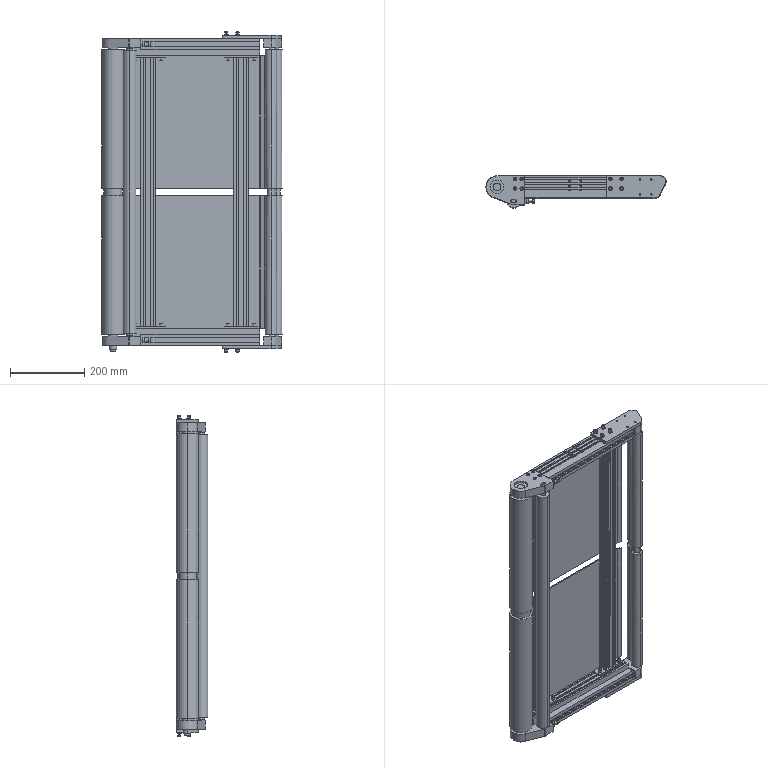Part | SolidWorks | features ICE 76, Revolution 36, RefAxis 18, RevCut 18, LPattern 16, 3DProfileFeature 6, CombineBodies 1, MoveCopyBody 1, MoveFace 1, Scale 1 | 1 solid | 1588 faces | box 485 x 86 x 861 mm | volume 7022086 mm3 | plane 1090 | cylinder 364 | spline 68 | cone 66 | commonest cylinder face diameters 5 x116 8.5 x48 10 x40 12 x20 4.134 x16 9.2 x16